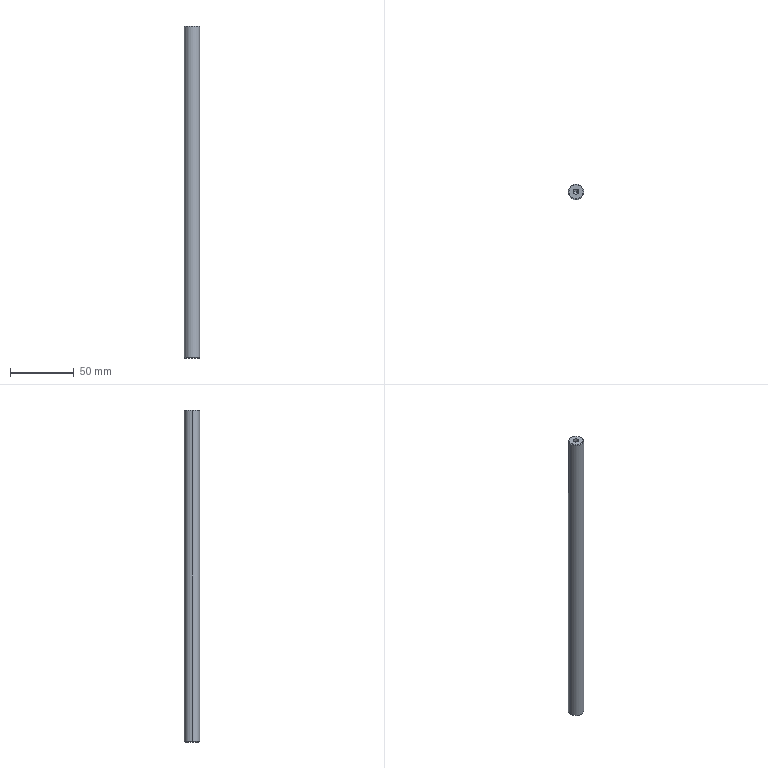Part | STEP file | 11-FG-S00111 | 1 solid | 12 faces | box 12 x 12 x 260 mm | volume 29196 mm3 | cone 6 | cylinder 4 | plane 2 | commonest cylinder face diameters 4.2 x2 12 x2
STEP:
#1=CARTESIAN_POINT('',(-5.5,0.,-130.));
#2=VERTEX_POINT('',#1);
#3=CARTESIAN_POINT('',(5.5,0.,-130.));
#4=VERTEX_POINT('',#3);
#5=CARTESIAN_POINT('',(0.,0.,-130.));
#6=DIRECTION('',(0.,0.,-1.));
#7=DIRECTION('',(1.,0.,0.));
#8=AXIS2_PLACEMENT_3D('',#5,#6,#7);
#9=CIRCLE('',#8,5.5);
#10=EDGE_CURVE('',#2,#4,#9,.T.);
#11=ORIENTED_EDGE('',*,*,#10,.F.);
#12=CARTESIAN_POINT('',(-6.,0.,-129.5));
#13=VERTEX_POINT('',#12);
#14=CARTESIAN_POINT('',(-6.,0.,-129.5));
#15=DIRECTION('',(-0.7071,0.,0.7071));
#16=VECTOR('',#15,1000.);
#17=LINE('',#14,#16);
#18=EDGE_CURVE('',#2,#13,#17,.T.);
#19=ORIENTED_EDGE('',*,*,#18,.T.);
#20=CARTESIAN_POINT('',(6.,0.,-129.5));
#21=VERTEX_POINT('',#20);
#22=CARTESIAN_POINT('',(0.,0.,-129.5));
#23=DIRECTION('',(0.,0.,1.));
#24=DIRECTION('',(1.,0.,0.));
#25=AXIS2_PLACEMENT_3D('',#22,#23,#24);
#26=CIRCLE('',#25,6.);
#27=EDGE_CURVE('',#21,#13,#26,.T.);
#28=ORIENTED_EDGE('',*,*,#27,.F.);
#29=CARTESIAN_POINT('',(6.,0.,-129.5));
#30=DIRECTION('',(0.7071,0.,0.7071));
#31=VECTOR('',#30,1000.);
#32=LINE('',#29,#31);
#33=EDGE_CURVE('',#4,#21,#32,.T.);
#34=ORIENTED_EDGE('',*,*,#33,.F.);
#35=EDGE_LOOP('',(#11,#19,#28,#34));
#36=FACE_OUTER_BOUND('',#35,.T.);
#37=CARTESIAN_POINT('',(0.,0.,-129.5));
#38=DIRECTION('',(0.,0.,1.));
#39=DIRECTION('',(1.,0.,0.));
#40=AXIS2_PLACEMENT_3D('',#37,#38,#39);
#41=CONICAL_SURFACE('',#40,6.,0.7854);
#42=ADVANCED_FACE('',(#36),#41,.T.);
#43=CARTESIAN_POINT('',(5.5,0.,130.));
#44=VERTEX_POINT('',#43);
#45=CARTESIAN_POINT('',(-5.5,0.,130.));
#46=VERTEX_POINT('',#45);
#47=CARTESIAN_POINT('',(0.,0.,130.));
#48=DIRECTION('',(0.,0.,1.));
#49=DIRECTION('',(1.,0.,0.));
#50=AXIS2_PLACEMENT_3D('',#47,#48,#49);
#51=CIRCLE('',#50,5.5);
#52=EDGE_CURVE('',#44,#46,#51,.T.);
#53=ORIENTED_EDGE('',*,*,#52,.F.);
#54=CARTESIAN_POINT('',(6.,0.,129.5));
#55=VERTEX_POINT('',#54);
#56=CARTESIAN_POINT('',(5.5,0.,130.));
#57=DIRECTION('',(0.7071,0.,-0.7071));
#58=VECTOR('',#57,1000.);
#59=LINE('',#56,#58);
#60=EDGE_CURVE('',#44,#55,#59,.T.);
#61=ORIENTED_EDGE('',*,*,#60,.T.);
#62=CARTESIAN_POINT('',(-6.,0.,129.5));
#63=VERTEX_POINT('',#62);
#64=CARTESIAN_POINT('',(0.,0.,129.5));
#65=DIRECTION('',(0.,0.,-1.));
#66=DIRECTION('',(1.,0.,0.));
#67=AXIS2_PLACEMENT_3D('',#64,#65,#66);
#68=CIRCLE('',#67,6.);
#69=EDGE_CURVE('',#63,#55,#68,.T.);
#70=ORIENTED_EDGE('',*,*,#69,.F.);
#71=CARTESIAN_POINT('',(-5.5,0.,130.));
#72=DIRECTION('',(-0.7071,0.,-0.7071));
#73=VECTOR('',#72,1000.);
#74=LINE('',#71,#73);
#75=EDGE_CURVE('',#46,#63,#74,.T.);
#76=ORIENTED_EDGE('',*,*,#75,.F.);
#77=EDGE_LOOP('',(#53,#61,#70,#76));
#78=FACE_OUTER_BOUND('',#77,.T.);
#79=CARTESIAN_POINT('',(0.,0.,130.));
#80=DIRECTION('',(0.,0.,-1.));
#81=DIRECTION('',(-1.,0.,0.));
#82=AXIS2_PLACEMENT_3D('',#79,#80,#81);
#83=CONICAL_SURFACE('',#82,5.5,0.7854);
#84=ADVANCED_FACE('',(#78),#83,.T.);
#85=CARTESIAN_POINT('',(-2.1,0.,116.));
#86=VERTEX_POINT('',#85);
#87=CARTESIAN_POINT('',(2.1,0.,116.));
#88=VERTEX_POINT('',#87);
#89=CARTESIAN_POINT('',(0.,0.,116.));
#90=DIRECTION('',(0.,0.,1.));
#91=DIRECTION('',(1.,0.,0.));
#92=AXIS2_PLACEMENT_3D('',#89,#90,#91);
#93=CIRCLE('',#92,2.1);
#94=EDGE_CURVE('',#86,#88,#93,.T.);
#95=ORIENTED_EDGE('',*,*,#94,.F.);
#96=CARTESIAN_POINT('',(-2.1,0.,130.));
#97=VERTEX_POINT('',#96);
#98=CARTESIAN_POINT('',(-2.1,0.,130.));
#99=DIRECTION('',(0.,0.,1.));
#100=VECTOR('',#99,1000.);
#101=LINE('',#98,#100);
#102=EDGE_CURVE('',#86,#97,#101,.T.);
#103=ORIENTED_EDGE('',*,*,#102,.T.);
#104=CARTESIAN_POINT('',(2.1,0.,130.));
#105=VERTEX_POINT('',#104);
#106=CARTESIAN_POINT('',(0.,0.,130.));
#107=DIRECTION('',(0.,0.,1.));
#108=DIRECTION('',(1.,0.,0.));
#109=AXIS2_PLACEMENT_3D('',#106,#107,#108);
#110=CIRCLE('',#109,2.1);
#111=EDGE_CURVE('',#97,#105,#110,.T.);
#112=ORIENTED_EDGE('',*,*,#111,.T.);
#113=CARTESIAN_POINT('',(2.1,0.,130.));
#114=DIRECTION('',(0.,0.,1.));
#115=VECTOR('',#114,1000.);
#116=LINE('',#113,#115);
#117=EDGE_CURVE('',#88,#105,#116,.T.);
#118=ORIENTED_EDGE('',*,*,#117,.F.);
#119=EDGE_LOOP('',(#95,#103,#112,#118));
#120=FACE_OUTER_BOUND('',#119,.T.);
#121=CARTESIAN_POINT('',(0.,0.,130.));
#122=DIRECTION('',(0.,0.,1.));
#123=DIRECTION('',(1.,0.,0.));
#124=AXIS2_PLACEMENT_3D('',#121,#122,#123);
#125=CYLINDRICAL_SURFACE('',#124,2.1);
#126=ADVANCED_FACE('',(#120),#125,.F.);
#127=CARTESIAN_POINT('',(0.,0.,114.738));
#128=VERTEX_POINT('',#127);
#129=CARTESIAN_POINT('',(2.1,0.,116.));
#130=DIRECTION('',(0.8572,0.,0.515));
#131=VECTOR('',#130,1000.);
#132=LINE('',#129,#131);
#133=EDGE_CURVE('',#128,#88,#132,.T.);
#134=ORIENTED_EDGE('',*,*,#133,.F.);
#135=CARTESIAN_POINT('',(-2.1,0.,116.));
#136=DIRECTION('',(-0.8572,0.,0.515));
#137=VECTOR('',#136,1000.);
#138=LINE('',#135,#137);
#139=EDGE_CURVE('',#128,#86,#138,.T.);
#140=ORIENTED_EDGE('',*,*,#139,.T.);
#141=ORIENTED_EDGE('',*,*,#94,.T.);
#142=EDGE_LOOP('',(#134,#140,#141));
#143=FACE_OUTER_BOUND('',#142,.T.);
#144=CARTESIAN_POINT('',(0.,0.,116.));
#145=DIRECTION('',(0.,0.,1.));
#146=DIRECTION('',(1.,0.,0.));
#147=AXIS2_PLACEMENT_3D('',#144,#145,#146);
#148=CONICAL_SURFACE('',#147,2.1,1.03);
#149=ADVANCED_FACE('',(#143),#148,.F.);
#150=ORIENTED_EDGE('',*,*,#69,.T.);
#151=CARTESIAN_POINT('',(6.,0.,130.));
#152=DIRECTION('',(0.,0.,-1.));
#153=VECTOR('',#152,1000.);
#154=LINE('',#151,#153);
#155=EDGE_CURVE('',#55,#21,#154,.T.);
#156=ORIENTED_EDGE('',*,*,#155,.T.);
#157=ORIENTED_EDGE('',*,*,#27,.T.);
#158=CARTESIAN_POINT('',(-6.,0.,130.));
#159=DIRECTION('',(0.,0.,-1.));
#160=VECTOR('',#159,1000.);
#161=LINE('',#158,#160);
#162=EDGE_CURVE('',#63,#13,#161,.T.);
#163=ORIENTED_EDGE('',*,*,#162,.F.);
#164=EDGE_LOOP('',(#150,#156,#157,#163));
#165=FACE_OUTER_BOUND('',#164,.T.);
#166=CARTESIAN_POINT('',(0.,0.,130.));
#167=DIRECTION('',(0.,0.,-1.));
#168=DIRECTION('',(-1.,0.,0.));
#169=AXIS2_PLACEMENT_3D('',#166,#167,#168);
#170=CYLINDRICAL_SURFACE('',#169,6.);
#171=ADVANCED_FACE('',(#165),#170,.T.);
#172=ORIENTED_EDGE('',*,*,#155,.F.);
#173=CARTESIAN_POINT('',(0.,0.,129.5));
#174=DIRECTION('',(0.,0.,-1.));
#175=DIRECTION('',(1.,0.,0.));
#176=AXIS2_PLACEMENT_3D('',#173,#174,#175);
#177=CIRCLE('',#176,6.);
#178=EDGE_CURVE('',#55,#63,#177,.T.);
#179=ORIENTED_EDGE('',*,*,#178,.T.);
#180=ORIENTED_EDGE('',*,*,#162,.T.);
#181=CARTESIAN_POINT('',(0.,0.,-129.5));
#182=DIRECTION('',(0.,0.,1.));
#183=DIRECTION('',(1.,0.,0.));
#184=AXIS2_PLACEMENT_3D('',#181,#182,#183);
#185=CIRCLE('',#184,6.);
#186=EDGE_CURVE('',#13,#21,#185,.T.);
#187=ORIENTED_EDGE('',*,*,#186,.T.);
#188=EDGE_LOOP('',(#172,#179,#180,#187));
#189=FACE_OUTER_BOUND('',#188,.T.);
#190=CARTESIAN_POINT('',(0.,0.,130.));
#191=DIRECTION('',(0.,0.,-1.));
#192=DIRECTION('',(-1.,0.,0.));
#193=AXIS2_PLACEMENT_3D('',#190,#191,#192);
#194=CYLINDRICAL_SURFACE('',#193,6.);
#195=ADVANCED_FACE('',(#189),#194,.T.);
#196=CARTESIAN_POINT('',(0.,0.,130.));
#197=DIRECTION('',(0.,0.,1.));
#198=DIRECTION('',(1.,0.,0.));
#199=AXIS2_PLACEMENT_3D('',#196,#197,#198);
#200=CIRCLE('',#199,5.5);
#201=EDGE_CURVE('',#46,#44,#200,.T.);
#202=ORIENTED_EDGE('',*,*,#201,.T.);
#203=ORIENTED_EDGE('',*,*,#52,.T.);
#204=EDGE_LOOP('',(#202,#203));
#205=FACE_OUTER_BOUND('',#204,.T.);
#206=CARTESIAN_POINT('',(0.,0.,130.));
#207=DIRECTION('',(0.,0.,1.));
#208=DIRECTION('',(1.,0.,0.));
#209=AXIS2_PLACEMENT_3D('',#206,#207,#208);
#210=CIRCLE('',#209,2.1);
#211=EDGE_CURVE('',#105,#97,#210,.T.);
#212=ORIENTED_EDGE('',*,*,#211,.F.);
#213=ORIENTED_EDGE('',*,*,#111,.F.);
#214=EDGE_LOOP('',(#212,#213));
#215=FACE_BOUND('',#214,.T.);
#216=CARTESIAN_POINT('',(0.,0.,130.));
#217=DIRECTION('',(0.,0.,1.));
#218=DIRECTION('',(1.,0.,0.));
#219=AXIS2_PLACEMENT_3D('',#216,#217,#218);
#220=PLANE('',#219);
#221=ADVANCED_FACE('',(#205,#215),#220,.T.);
#222=CARTESIAN_POINT('',(0.,0.,-130.));
#223=DIRECTION('',(0.,0.,-1.));
#224=DIRECTION('',(1.,0.,0.));
#225=AXIS2_PLACEMENT_3D('',#222,#223,#224);
#226=CIRCLE('',#225,5.5);
#227=EDGE_CURVE('',#4,#2,#226,.T.);
#228=ORIENTED_EDGE('',*,*,#227,.T.);
#229=ORIENTED_EDGE('',*,*,#10,.T.);
#230=EDGE_LOOP('',(#228,#229));
#231=FACE_OUTER_BOUND('',#230,.T.);
#232=CARTESIAN_POINT('',(0.,0.,-130.));
#233=DIRECTION('',(0.,0.,1.));
#234=DIRECTION('',(1.,0.,0.));
#235=AXIS2_PLACEMENT_3D('',#232,#233,#234);
#236=PLANE('',#235);
#237=ADVANCED_FACE('',(#231),#236,.F.);
#238=ORIENTED_EDGE('',*,*,#139,.F.);
#239=ORIENTED_EDGE('',*,*,#133,.T.);
#240=CARTESIAN_POINT('',(0.,0.,116.));
#241=DIRECTION('',(0.,0.,1.));
#242=DIRECTION('',(1.,0.,0.));
#243=AXIS2_PLACEMENT_3D('',#240,#241,#242);
#244=CIRCLE('',#243,2.1);
#245=EDGE_CURVE('',#88,#86,#244,.T.);
#246=ORIENTED_EDGE('',*,*,#245,.T.);
#247=EDGE_LOOP('',(#238,#239,#246));
#248=FACE_OUTER_BOUND('',#247,.T.);
#249=CARTESIAN_POINT('',(0.,0.,116.));
#250=DIRECTION('',(0.,0.,1.));
#251=DIRECTION('',(1.,0.,0.));
#252=AXIS2_PLACEMENT_3D('',#249,#250,#251);
#253=CONICAL_SURFACE('',#252,2.1,1.03);
#254=ADVANCED_FACE('',(#248),#253,.F.);
#255=ORIENTED_EDGE('',*,*,#102,.F.);
#256=ORIENTED_EDGE('',*,*,#245,.F.);
#257=ORIENTED_EDGE('',*,*,#117,.T.);
#258=ORIENTED_EDGE('',*,*,#211,.T.);
#259=EDGE_LOOP('',(#255,#256,#257,#258));
#260=FACE_OUTER_BOUND('',#259,.T.);
#261=CARTESIAN_POINT('',(0.,0.,130.));
#262=DIRECTION('',(0.,0.,1.));
#263=DIRECTION('',(1.,0.,0.));
#264=AXIS2_PLACEMENT_3D('',#261,#262,#263);
#265=CYLINDRICAL_SURFACE('',#264,2.1);
#266=ADVANCED_FACE('',(#260),#265,.F.);
#267=ORIENTED_EDGE('',*,*,#60,.F.);
#268=ORIENTED_EDGE('',*,*,#201,.F.);
#269=ORIENTED_EDGE('',*,*,#75,.T.);
#270=ORIENTED_EDGE('',*,*,#178,.F.);
#271=EDGE_LOOP('',(#267,#268,#269,#270));
#272=FACE_OUTER_BOUND('',#271,.T.);
#273=CARTESIAN_POINT('',(0.,0.,130.));
#274=DIRECTION('',(0.,0.,-1.));
#275=DIRECTION('',(-1.,0.,0.));
#276=AXIS2_PLACEMENT_3D('',#273,#274,#275);
#277=CONICAL_SURFACE('',#276,5.5,0.7854);
#278=ADVANCED_FACE('',(#272),#277,.T.);
#279=ORIENTED_EDGE('',*,*,#18,.F.);
#280=ORIENTED_EDGE('',*,*,#227,.F.);
#281=ORIENTED_EDGE('',*,*,#33,.T.);
#282=ORIENTED_EDGE('',*,*,#186,.F.);
#283=EDGE_LOOP('',(#279,#280,#281,#282));
#284=FACE_OUTER_BOUND('',#283,.T.);
#285=CARTESIAN_POINT('',(0.,0.,-129.5));
#286=DIRECTION('',(0.,0.,1.));
#287=DIRECTION('',(1.,0.,0.));
#288=AXIS2_PLACEMENT_3D('',#285,#286,#287);
#289=CONICAL_SURFACE('',#288,6.,0.7854);
#290=ADVANCED_FACE('',(#284),#289,.T.);
#291=CLOSED_SHELL('',(#42,#84,#126,#149,#171,#195,#221,#237,#254,#266,#278,#290));
#292=MANIFOLD_SOLID_BREP('',#291);
#293=CARTESIAN_POINT('',(0.,0.,0.));
#294=DIRECTION('',(0.,0.,1.));
#295=DIRECTION('',(1.,0.,0.));
#296=AXIS2_PLACEMENT_3D('',#293,#294,#295);
#297=(LENGTH_UNIT()NAMED_UNIT(*)SI_UNIT(.MILLI.,.METRE.));
#298=UNCERTAINTY_MEASURE_WITH_UNIT(LENGTH_MEASURE(0.00001),#297,'','');
#299=(NAMED_UNIT(*)PLANE_ANGLE_UNIT()SI_UNIT($,.RADIAN.));
#300=(NAMED_UNIT(*)SI_UNIT($,.STERADIAN.)SOLID_ANGLE_UNIT());
#301=(GEOMETRIC_REPRESENTATION_CONTEXT(3)GLOBAL_UNCERTAINTY_ASSIGNED_CONTEXT((#298))GLOBAL_UNIT_ASSIGNED_CONTEXT((#297,#299,#300))REPRESENTATION_CONTEXT('',''));
#302=ADVANCED_BREP_SHAPE_REPRESENTATION('',(#292,#296),#301);